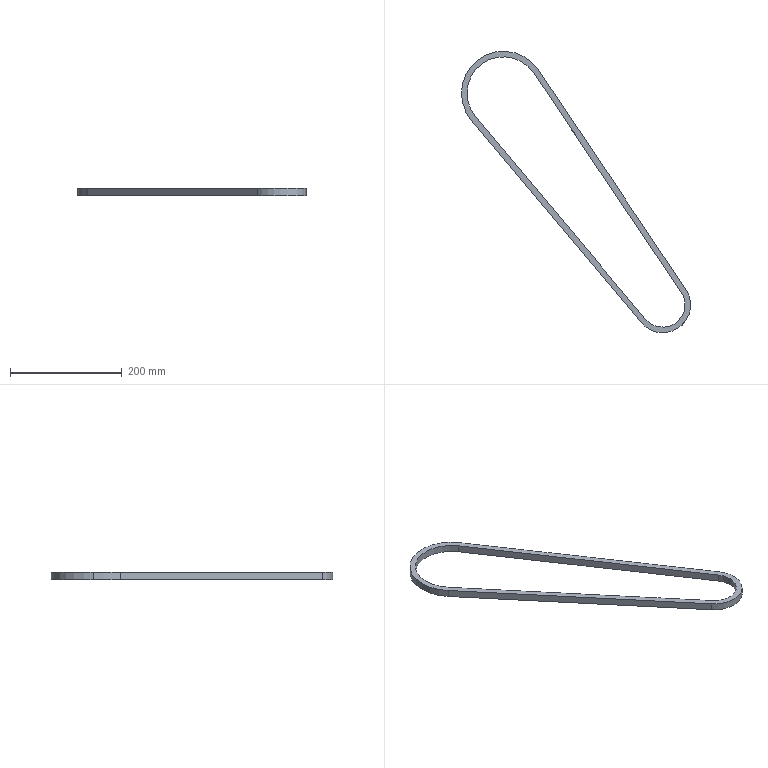Part | SolidWorks | features BeltProfileFeature 1, ExtruThin 1 | 1 solid | 12 faces | box 410 x 503.461 x 13 mm | volume 170318 mm3 | cylinder 6 | plane 6 | commonest cylinder face diameters 130 x2 150 x2 80 x1 100 x1
STEP:
#1=CARTESIAN_POINT('',(-65.,0.,6.5));
#2=VERTEX_POINT('',#1);
#3=CARTESIAN_POINT('',(53.915,36.307,6.5));
#4=VERTEX_POINT('',#3);
#5=CARTESIAN_POINT('',(0.,0.,6.5));
#6=DIRECTION('',(0.,0.,-1.));
#7=DIRECTION('',(-1.,0.,0.));
#8=AXIS2_PLACEMENT_3D('',#5,#6,#7);
#9=CIRCLE('',#8,65.);
#10=EDGE_CURVE('',#2,#4,#9,.T.);
#11=ORIENTED_EDGE('',*,*,#10,.F.);
#12=CARTESIAN_POINT('',(-65.,0.,-6.5));
#13=VERTEX_POINT('',#12);
#14=CARTESIAN_POINT('',(-65.,0.,6.5));
#15=DIRECTION('',(0.,0.,-1.));
#16=VECTOR('',#15,1000.);
#17=LINE('',#14,#16);
#18=EDGE_CURVE('',#2,#13,#17,.T.);
#19=ORIENTED_EDGE('',*,*,#18,.T.);
#20=CARTESIAN_POINT('',(53.915,36.307,-6.5));
#21=VERTEX_POINT('',#20);
#22=CARTESIAN_POINT('',(0.,0.,-6.5));
#23=DIRECTION('',(0.,0.,-1.));
#24=DIRECTION('',(-1.,0.,0.));
#25=AXIS2_PLACEMENT_3D('',#22,#23,#24);
#26=CIRCLE('',#25,65.);
#27=EDGE_CURVE('',#13,#21,#26,.T.);
#28=ORIENTED_EDGE('',*,*,#27,.T.);
#29=CARTESIAN_POINT('',(53.915,36.307,6.5));
#30=DIRECTION('',(0.,0.,-1.));
#31=VECTOR('',#30,1000.);
#32=LINE('',#29,#31);
#33=EDGE_CURVE('',#4,#21,#32,.T.);
#34=ORIENTED_EDGE('',*,*,#33,.F.);
#35=EDGE_LOOP('',(#11,#19,#28,#34));
#36=FACE_OUTER_BOUND('',#35,.T.);
#37=CARTESIAN_POINT('',(0.,0.,6.5));
#38=DIRECTION('',(0.,0.,-1.));
#39=DIRECTION('',(-1.,0.,0.));
#40=AXIS2_PLACEMENT_3D('',#37,#38,#39);
#41=CYLINDRICAL_SURFACE('',#40,65.);
#42=ADVANCED_FACE('',(#36),#41,.F.);
#43=CARTESIAN_POINT('',(-57.448,-48.215,6.5));
#44=VERTEX_POINT('',#43);
#45=CARTESIAN_POINT('',(-75.,0.,6.5));
#46=VERTEX_POINT('',#45);
#47=CARTESIAN_POINT('',(0.,0.,6.5));
#48=DIRECTION('',(0.,0.,-1.));
#49=DIRECTION('',(-1.,0.,0.));
#50=AXIS2_PLACEMENT_3D('',#47,#48,#49);
#51=CIRCLE('',#50,75.);
#52=EDGE_CURVE('',#44,#46,#51,.T.);
#53=ORIENTED_EDGE('',*,*,#52,.T.);
#54=CARTESIAN_POINT('',(-75.,0.,-6.5));
#55=VERTEX_POINT('',#54);
#56=CARTESIAN_POINT('',(-75.,0.,6.5));
#57=DIRECTION('',(0.,0.,-1.));
#58=VECTOR('',#57,1000.);
#59=LINE('',#56,#58);
#60=EDGE_CURVE('',#46,#55,#59,.T.);
#61=ORIENTED_EDGE('',*,*,#60,.T.);
#62=CARTESIAN_POINT('',(-57.448,-48.215,-6.5));
#63=VERTEX_POINT('',#62);
#64=CARTESIAN_POINT('',(0.,0.,-6.5));
#65=DIRECTION('',(0.,0.,-1.));
#66=DIRECTION('',(-1.,0.,0.));
#67=AXIS2_PLACEMENT_3D('',#64,#65,#66);
#68=CIRCLE('',#67,75.);
#69=EDGE_CURVE('',#63,#55,#68,.T.);
#70=ORIENTED_EDGE('',*,*,#69,.F.);
#71=CARTESIAN_POINT('',(-57.448,-48.215,6.5));
#72=DIRECTION('',(0.,0.,-1.));
#73=VECTOR('',#72,1000.);
#74=LINE('',#71,#73);
#75=EDGE_CURVE('',#44,#63,#74,.T.);
#76=ORIENTED_EDGE('',*,*,#75,.F.);
#77=EDGE_LOOP('',(#53,#61,#70,#76));
#78=FACE_OUTER_BOUND('',#77,.T.);
#79=CARTESIAN_POINT('',(0.,0.,6.5));
#80=DIRECTION('',(0.,0.,-1.));
#81=DIRECTION('',(-1.,0.,0.));
#82=AXIS2_PLACEMENT_3D('',#79,#80,#81);
#83=CYLINDRICAL_SURFACE('',#82,75.);
#84=ADVANCED_FACE('',(#78),#83,.T.);
#85=CARTESIAN_POINT('',(246.701,-410.604,-6.5));
#86=VERTEX_POINT('',#85);
#87=CARTESIAN_POINT('',(246.701,-410.604,-6.5));
#88=DIRECTION('',(-0.6429,0.766,0.));
#89=VECTOR('',#88,1000.);
#90=LINE('',#87,#89);
#91=EDGE_CURVE('',#86,#63,#90,.T.);
#92=ORIENTED_EDGE('',*,*,#91,.F.);
#93=CARTESIAN_POINT('',(246.701,-410.604,6.5));
#94=VERTEX_POINT('',#93);
#95=CARTESIAN_POINT('',(246.701,-410.604,6.5));
#96=DIRECTION('',(0.,0.,-1.));
#97=VECTOR('',#96,1000.);
#98=LINE('',#95,#97);
#99=EDGE_CURVE('',#94,#86,#98,.T.);
#100=ORIENTED_EDGE('',*,*,#99,.F.);
#101=CARTESIAN_POINT('',(246.701,-410.604,6.5));
#102=DIRECTION('',(-0.6429,0.766,0.));
#103=VECTOR('',#102,1000.);
#104=LINE('',#101,#103);
#105=EDGE_CURVE('',#94,#44,#104,.T.);
#106=ORIENTED_EDGE('',*,*,#105,.T.);
#107=ORIENTED_EDGE('',*,*,#75,.T.);
#108=EDGE_LOOP('',(#92,#100,#106,#107));
#109=FACE_OUTER_BOUND('',#108,.T.);
#110=CARTESIAN_POINT('',(246.701,-410.604,6.5));
#111=DIRECTION('',(-0.766,-0.6429,0.));
#112=DIRECTION('',(0.6429,-0.766,0.));
#113=AXIS2_PLACEMENT_3D('',#110,#111,#112);
#114=PLANE('',#113);
#115=ADVANCED_FACE('',(#109),#114,.T.);
#116=CARTESIAN_POINT('',(326.473,-350.532,-6.5));
#117=VERTEX_POINT('',#116);
#118=CARTESIAN_POINT('',(285.,-378.461,-6.5));
#119=DIRECTION('',(0.,0.,-1.));
#120=DIRECTION('',(-1.,0.,0.));
#121=AXIS2_PLACEMENT_3D('',#118,#119,#120);
#122=CIRCLE('',#121,50.);
#123=EDGE_CURVE('',#117,#86,#122,.T.);
#124=ORIENTED_EDGE('',*,*,#123,.F.);
#125=CARTESIAN_POINT('',(326.473,-350.532,6.5));
#126=VERTEX_POINT('',#125);
#127=CARTESIAN_POINT('',(326.473,-350.532,6.5));
#128=DIRECTION('',(0.,0.,-1.));
#129=VECTOR('',#128,1000.);
#130=LINE('',#127,#129);
#131=EDGE_CURVE('',#126,#117,#130,.T.);
#132=ORIENTED_EDGE('',*,*,#131,.F.);
#133=CARTESIAN_POINT('',(285.,-378.461,6.5));
#134=DIRECTION('',(0.,0.,-1.));
#135=DIRECTION('',(-1.,0.,0.));
#136=AXIS2_PLACEMENT_3D('',#133,#134,#135);
#137=CIRCLE('',#136,50.);
#138=EDGE_CURVE('',#126,#94,#137,.T.);
#139=ORIENTED_EDGE('',*,*,#138,.T.);
#140=ORIENTED_EDGE('',*,*,#99,.T.);
#141=EDGE_LOOP('',(#124,#132,#139,#140));
#142=FACE_OUTER_BOUND('',#141,.T.);
#143=CARTESIAN_POINT('',(285.,-378.461,6.5));
#144=DIRECTION('',(0.,0.,-1.));
#145=DIRECTION('',(-1.,0.,0.));
#146=AXIS2_PLACEMENT_3D('',#143,#144,#145);
#147=CYLINDRICAL_SURFACE('',#146,50.);
#148=ADVANCED_FACE('',(#142),#147,.T.);
#149=CARTESIAN_POINT('',(62.209,41.893,-6.5));
#150=VERTEX_POINT('',#149);
#151=CARTESIAN_POINT('',(62.209,41.893,-6.5));
#152=DIRECTION('',(0.5586,-0.8295,0.));
#153=VECTOR('',#152,1000.);
#154=LINE('',#151,#153);
#155=EDGE_CURVE('',#150,#117,#154,.T.);
#156=ORIENTED_EDGE('',*,*,#155,.F.);
#157=CARTESIAN_POINT('',(62.209,41.893,6.5));
#158=VERTEX_POINT('',#157);
#159=CARTESIAN_POINT('',(62.209,41.893,6.5));
#160=DIRECTION('',(0.,0.,-1.));
#161=VECTOR('',#160,1000.);
#162=LINE('',#159,#161);
#163=EDGE_CURVE('',#158,#150,#162,.T.);
#164=ORIENTED_EDGE('',*,*,#163,.F.);
#165=CARTESIAN_POINT('',(62.209,41.893,6.5));
#166=DIRECTION('',(0.5586,-0.8295,0.));
#167=VECTOR('',#166,1000.);
#168=LINE('',#165,#167);
#169=EDGE_CURVE('',#158,#126,#168,.T.);
#170=ORIENTED_EDGE('',*,*,#169,.T.);
#171=ORIENTED_EDGE('',*,*,#131,.T.);
#172=EDGE_LOOP('',(#156,#164,#170,#171));
#173=FACE_OUTER_BOUND('',#172,.T.);
#174=CARTESIAN_POINT('',(62.209,41.893,6.5));
#175=DIRECTION('',(0.8295,0.5586,0.));
#176=DIRECTION('',(-0.5586,0.8295,0.));
#177=AXIS2_PLACEMENT_3D('',#174,#175,#176);
#178=PLANE('',#177);
#179=ADVANCED_FACE('',(#173),#178,.T.);
#180=ORIENTED_EDGE('',*,*,#60,.F.);
#181=CARTESIAN_POINT('',(0.,0.,6.5));
#182=DIRECTION('',(0.,0.,-1.));
#183=DIRECTION('',(-1.,0.,0.));
#184=AXIS2_PLACEMENT_3D('',#181,#182,#183);
#185=CIRCLE('',#184,75.);
#186=EDGE_CURVE('',#46,#158,#185,.T.);
#187=ORIENTED_EDGE('',*,*,#186,.T.);
#188=ORIENTED_EDGE('',*,*,#163,.T.);
#189=CARTESIAN_POINT('',(0.,0.,-6.5));
#190=DIRECTION('',(0.,0.,-1.));
#191=DIRECTION('',(-1.,0.,0.));
#192=AXIS2_PLACEMENT_3D('',#189,#190,#191);
#193=CIRCLE('',#192,75.);
#194=EDGE_CURVE('',#55,#150,#193,.T.);
#195=ORIENTED_EDGE('',*,*,#194,.F.);
#196=EDGE_LOOP('',(#180,#187,#188,#195));
#197=FACE_OUTER_BOUND('',#196,.T.);
#198=CARTESIAN_POINT('',(0.,0.,6.5));
#199=DIRECTION('',(0.,0.,-1.));
#200=DIRECTION('',(-1.,0.,0.));
#201=AXIS2_PLACEMENT_3D('',#198,#199,#200);
#202=CYLINDRICAL_SURFACE('',#201,75.);
#203=ADVANCED_FACE('',(#197),#202,.T.);
#204=CARTESIAN_POINT('',(318.178,-356.118,6.5));
#205=VERTEX_POINT('',#204);
#206=CARTESIAN_POINT('',(254.361,-404.176,6.5));
#207=VERTEX_POINT('',#206);
#208=CARTESIAN_POINT('',(285.,-378.461,6.5));
#209=DIRECTION('',(0.,0.,-1.));
#210=DIRECTION('',(-1.,0.,0.));
#211=AXIS2_PLACEMENT_3D('',#208,#209,#210);
#212=CIRCLE('',#211,40.);
#213=EDGE_CURVE('',#205,#207,#212,.T.);
#214=ORIENTED_EDGE('',*,*,#213,.T.);
#215=CARTESIAN_POINT('',(-49.788,-41.787,6.5));
#216=VERTEX_POINT('',#215);
#217=CARTESIAN_POINT('',(-49.788,-41.787,6.5));
#218=DIRECTION('',(-0.6429,0.766,0.));
#219=VECTOR('',#218,1000.);
#220=LINE('',#217,#219);
#221=EDGE_CURVE('',#207,#216,#220,.T.);
#222=ORIENTED_EDGE('',*,*,#221,.T.);
#223=CARTESIAN_POINT('',(0.,0.,6.5));
#224=DIRECTION('',(0.,0.,-1.));
#225=DIRECTION('',(-1.,0.,0.));
#226=AXIS2_PLACEMENT_3D('',#223,#224,#225);
#227=CIRCLE('',#226,65.);
#228=EDGE_CURVE('',#216,#2,#227,.T.);
#229=ORIENTED_EDGE('',*,*,#228,.T.);
#230=ORIENTED_EDGE('',*,*,#10,.T.);
#231=CARTESIAN_POINT('',(53.915,36.307,6.5));
#232=DIRECTION('',(0.5586,-0.8295,0.));
#233=VECTOR('',#232,1000.);
#234=LINE('',#231,#233);
#235=EDGE_CURVE('',#4,#205,#234,.T.);
#236=ORIENTED_EDGE('',*,*,#235,.T.);
#237=EDGE_LOOP('',(#214,#222,#229,#230,#236));
#238=FACE_BOUND('',#237,.T.);
#239=ORIENTED_EDGE('',*,*,#105,.F.);
#240=ORIENTED_EDGE('',*,*,#138,.F.);
#241=ORIENTED_EDGE('',*,*,#169,.F.);
#242=ORIENTED_EDGE('',*,*,#186,.F.);
#243=ORIENTED_EDGE('',*,*,#52,.F.);
#244=EDGE_LOOP('',(#239,#240,#241,#242,#243));
#245=FACE_OUTER_BOUND('',#244,.T.);
#246=CARTESIAN_POINT('',(0.,0.,6.5));
#247=DIRECTION('',(0.,0.,-1.));
#248=DIRECTION('',(-1.,0.,0.));
#249=AXIS2_PLACEMENT_3D('',#246,#247,#248);
#250=PLANE('',#249);
#251=ADVANCED_FACE('',(#238,#245),#250,.F.);
#252=CARTESIAN_POINT('',(254.361,-404.176,-6.5));
#253=VERTEX_POINT('',#252);
#254=CARTESIAN_POINT('',(-49.788,-41.787,-6.5));
#255=VERTEX_POINT('',#254);
#256=CARTESIAN_POINT('',(-49.788,-41.787,-6.5));
#257=DIRECTION('',(-0.6429,0.766,0.));
#258=VECTOR('',#257,1000.);
#259=LINE('',#256,#258);
#260=EDGE_CURVE('',#253,#255,#259,.T.);
#261=ORIENTED_EDGE('',*,*,#260,.F.);
#262=CARTESIAN_POINT('',(318.178,-356.118,-6.5));
#263=VERTEX_POINT('',#262);
#264=CARTESIAN_POINT('',(285.,-378.461,-6.5));
#265=DIRECTION('',(0.,0.,-1.));
#266=DIRECTION('',(-1.,0.,0.));
#267=AXIS2_PLACEMENT_3D('',#264,#265,#266);
#268=CIRCLE('',#267,40.);
#269=EDGE_CURVE('',#263,#253,#268,.T.);
#270=ORIENTED_EDGE('',*,*,#269,.F.);
#271=CARTESIAN_POINT('',(53.915,36.307,-6.5));
#272=DIRECTION('',(0.5586,-0.8295,0.));
#273=VECTOR('',#272,1000.);
#274=LINE('',#271,#273);
#275=EDGE_CURVE('',#21,#263,#274,.T.);
#276=ORIENTED_EDGE('',*,*,#275,.F.);
#277=ORIENTED_EDGE('',*,*,#27,.F.);
#278=CARTESIAN_POINT('',(0.,0.,-6.5));
#279=DIRECTION('',(0.,0.,-1.));
#280=DIRECTION('',(-1.,0.,0.));
#281=AXIS2_PLACEMENT_3D('',#278,#279,#280);
#282=CIRCLE('',#281,65.);
#283=EDGE_CURVE('',#255,#13,#282,.T.);
#284=ORIENTED_EDGE('',*,*,#283,.F.);
#285=EDGE_LOOP('',(#261,#270,#276,#277,#284));
#286=FACE_BOUND('',#285,.T.);
#287=ORIENTED_EDGE('',*,*,#91,.T.);
#288=ORIENTED_EDGE('',*,*,#69,.T.);
#289=ORIENTED_EDGE('',*,*,#194,.T.);
#290=ORIENTED_EDGE('',*,*,#155,.T.);
#291=ORIENTED_EDGE('',*,*,#123,.T.);
#292=EDGE_LOOP('',(#287,#288,#289,#290,#291));
#293=FACE_OUTER_BOUND('',#292,.T.);
#294=CARTESIAN_POINT('',(0.,0.,-6.5));
#295=DIRECTION('',(0.,0.,-1.));
#296=DIRECTION('',(-1.,0.,0.));
#297=AXIS2_PLACEMENT_3D('',#294,#295,#296);
#298=PLANE('',#297);
#299=ADVANCED_FACE('',(#286,#293),#298,.T.);
#300=ORIENTED_EDGE('',*,*,#260,.T.);
#301=CARTESIAN_POINT('',(-49.788,-41.787,6.5));
#302=DIRECTION('',(0.,0.,-1.));
#303=VECTOR('',#302,1000.);
#304=LINE('',#301,#303);
#305=EDGE_CURVE('',#216,#255,#304,.T.);
#306=ORIENTED_EDGE('',*,*,#305,.F.);
#307=ORIENTED_EDGE('',*,*,#221,.F.);
#308=CARTESIAN_POINT('',(254.361,-404.176,6.5));
#309=DIRECTION('',(0.,0.,-1.));
#310=VECTOR('',#309,1000.);
#311=LINE('',#308,#310);
#312=EDGE_CURVE('',#207,#253,#311,.T.);
#313=ORIENTED_EDGE('',*,*,#312,.T.);
#314=EDGE_LOOP('',(#300,#306,#307,#313));
#315=FACE_OUTER_BOUND('',#314,.T.);
#316=CARTESIAN_POINT('',(-49.788,-41.787,6.5));
#317=DIRECTION('',(-0.766,-0.6429,0.));
#318=DIRECTION('',(0.6429,-0.766,0.));
#319=AXIS2_PLACEMENT_3D('',#316,#317,#318);
#320=PLANE('',#319);
#321=ADVANCED_FACE('',(#315),#320,.F.);
#322=ORIENTED_EDGE('',*,*,#269,.T.);
#323=ORIENTED_EDGE('',*,*,#312,.F.);
#324=ORIENTED_EDGE('',*,*,#213,.F.);
#325=CARTESIAN_POINT('',(318.178,-356.118,6.5));
#326=DIRECTION('',(0.,0.,-1.));
#327=VECTOR('',#326,1000.);
#328=LINE('',#325,#327);
#329=EDGE_CURVE('',#205,#263,#328,.T.);
#330=ORIENTED_EDGE('',*,*,#329,.T.);
#331=EDGE_LOOP('',(#322,#323,#324,#330));
#332=FACE_OUTER_BOUND('',#331,.T.);
#333=CARTESIAN_POINT('',(285.,-378.461,6.5));
#334=DIRECTION('',(0.,0.,-1.));
#335=DIRECTION('',(-1.,0.,0.));
#336=AXIS2_PLACEMENT_3D('',#333,#334,#335);
#337=CYLINDRICAL_SURFACE('',#336,40.);
#338=ADVANCED_FACE('',(#332),#337,.F.);
#339=ORIENTED_EDGE('',*,*,#275,.T.);
#340=ORIENTED_EDGE('',*,*,#329,.F.);
#341=ORIENTED_EDGE('',*,*,#235,.F.);
#342=ORIENTED_EDGE('',*,*,#33,.T.);
#343=EDGE_LOOP('',(#339,#340,#341,#342));
#344=FACE_OUTER_BOUND('',#343,.T.);
#345=CARTESIAN_POINT('',(53.915,36.307,6.5));
#346=DIRECTION('',(0.8295,0.5586,0.));
#347=DIRECTION('',(-0.5586,0.8295,0.));
#348=AXIS2_PLACEMENT_3D('',#345,#346,#347);
#349=PLANE('',#348);
#350=ADVANCED_FACE('',(#344),#349,.F.);
#351=ORIENTED_EDGE('',*,*,#18,.F.);
#352=ORIENTED_EDGE('',*,*,#228,.F.);
#353=ORIENTED_EDGE('',*,*,#305,.T.);
#354=ORIENTED_EDGE('',*,*,#283,.T.);
#355=EDGE_LOOP('',(#351,#352,#353,#354));
#356=FACE_OUTER_BOUND('',#355,.T.);
#357=CARTESIAN_POINT('',(0.,0.,6.5));
#358=DIRECTION('',(0.,0.,-1.));
#359=DIRECTION('',(-1.,0.,0.));
#360=AXIS2_PLACEMENT_3D('',#357,#358,#359);
#361=CYLINDRICAL_SURFACE('',#360,65.);
#362=ADVANCED_FACE('',(#356),#361,.F.);
#363=CLOSED_SHELL('',(#42,#84,#115,#148,#179,#203,#251,#299,#321,#338,#350,#362));
#364=MANIFOLD_SOLID_BREP('',#363);
#365=CARTESIAN_POINT('',(0.,0.,0.));
#366=DIRECTION('',(0.,0.,1.));
#367=DIRECTION('',(1.,0.,0.));
#368=AXIS2_PLACEMENT_3D('',#365,#366,#367);
#369=(LENGTH_UNIT()NAMED_UNIT(*)SI_UNIT(.MILLI.,.METRE.));
#370=UNCERTAINTY_MEASURE_WITH_UNIT(LENGTH_MEASURE(0.00001),#369,'','');
#371=(NAMED_UNIT(*)PLANE_ANGLE_UNIT()SI_UNIT($,.RADIAN.));
#372=(NAMED_UNIT(*)SI_UNIT($,.STERADIAN.)SOLID_ANGLE_UNIT());
#373=(GEOMETRIC_REPRESENTATION_CONTEXT(3)GLOBAL_UNCERTAINTY_ASSIGNED_CONTEXT((#370))GLOBAL_UNIT_ASSIGNED_CONTEXT((#369,#371,#372))REPRESENTATION_CONTEXT('',''));
#374=ADVANCED_BREP_SHAPE_REPRESENTATION('',(#364,#368),#373);